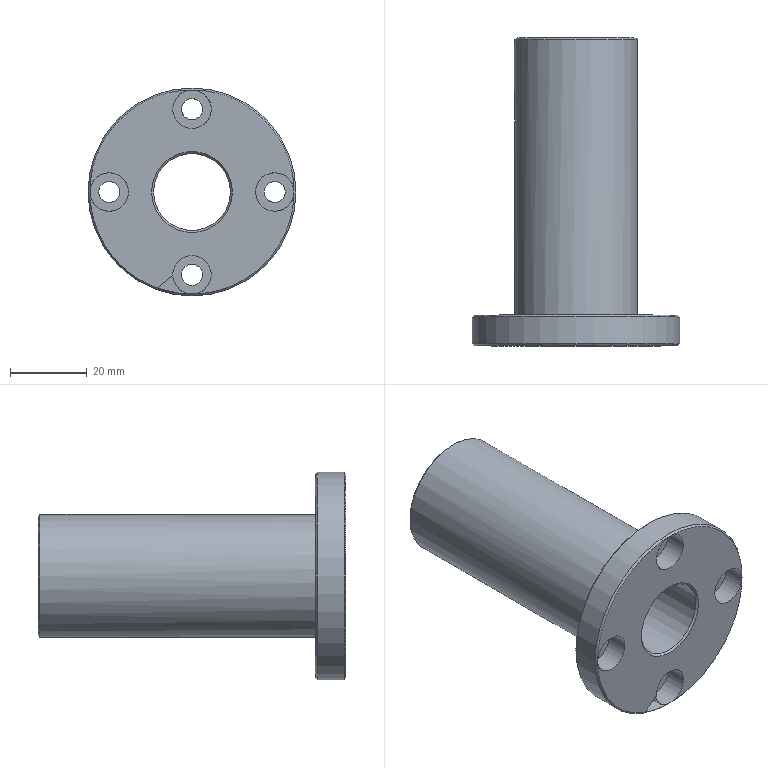Part | NX | 1 solid | 23 faces | box 54 x 80 x 54 mm | volume 49015 mm3 | cylinder 11 | plane 7 | cone 5 | commonest cylinder face diameters 5.5 x4 10 x4 20 x1 32 x1 54 x1
STEP:
#1=CARTESIAN_POINT('',(10.5,0.,0.));
#2=VERTEX_POINT('',#1);
#3=CARTESIAN_POINT('',(0.,0.,0.));
#4=DIRECTION('',(0.,-1.,0.));
#5=DIRECTION('',(1.,0.,0.));
#6=AXIS2_PLACEMENT_3D('',#3,#4,#5);
#7=CIRCLE('',#6,10.5);
#8=EDGE_CURVE('',#2,#2,#7,.F.);
#9=ORIENTED_EDGE('',*,*,#8,.T.);
#10=EDGE_LOOP('',(#9));
#11=FACE_BOUND('',#10,.T.);
#12=CARTESIAN_POINT('',(26.5,0.,0.));
#13=VERTEX_POINT('',#12);
#14=CARTESIAN_POINT('',(21.5,0.,0.));
#15=DIRECTION('',(0.,-1.,0.));
#16=DIRECTION('',(0.,0.,-1.));
#17=AXIS2_PLACEMENT_3D('',#14,#15,#16);
#18=CIRCLE('',#17,5.);
#19=EDGE_CURVE('',#13,#13,#18,.T.);
#20=ORIENTED_EDGE('',*,*,#19,.F.);
#21=CARTESIAN_POINT('',(0.,0.,26.5));
#22=VERTEX_POINT('',#21);
#23=CARTESIAN_POINT('',(0.,0.,0.));
#24=DIRECTION('',(0.,-1.,0.));
#25=DIRECTION('',(1.,0.,0.));
#26=AXIS2_PLACEMENT_3D('',#23,#24,#25);
#27=CIRCLE('',#26,26.5);
#28=EDGE_CURVE('',#13,#22,#27,.T.);
#29=ORIENTED_EDGE('',*,*,#28,.T.);
#30=CARTESIAN_POINT('',(0.,0.,21.5));
#31=DIRECTION('',(0.,-1.,0.));
#32=DIRECTION('',(0.,0.,-1.));
#33=AXIS2_PLACEMENT_3D('',#30,#31,#32);
#34=CIRCLE('',#33,5.);
#35=EDGE_CURVE('',#22,#22,#34,.T.);
#36=ORIENTED_EDGE('',*,*,#35,.F.);
#37=CARTESIAN_POINT('',(-26.5,0.,0.));
#38=VERTEX_POINT('',#37);
#39=CARTESIAN_POINT('',(0.,0.,0.));
#40=DIRECTION('',(0.,-1.,0.));
#41=DIRECTION('',(1.,0.,0.));
#42=AXIS2_PLACEMENT_3D('',#39,#40,#41);
#43=CIRCLE('',#42,26.5);
#44=EDGE_CURVE('',#22,#38,#43,.T.);
#45=ORIENTED_EDGE('',*,*,#44,.T.);
#46=CARTESIAN_POINT('',(-21.5,0.,0.));
#47=DIRECTION('',(0.,-1.,0.));
#48=DIRECTION('',(0.,0.,-1.));
#49=AXIS2_PLACEMENT_3D('',#46,#47,#48);
#50=CIRCLE('',#49,5.);
#51=EDGE_CURVE('',#38,#38,#50,.T.);
#52=ORIENTED_EDGE('',*,*,#51,.F.);
#53=CARTESIAN_POINT('',(0.,0.,-26.5));
#54=VERTEX_POINT('',#53);
#55=CARTESIAN_POINT('',(0.,0.,0.));
#56=DIRECTION('',(0.,-1.,0.));
#57=DIRECTION('',(1.,0.,0.));
#58=AXIS2_PLACEMENT_3D('',#55,#56,#57);
#59=CIRCLE('',#58,26.5);
#60=EDGE_CURVE('',#38,#54,#59,.T.);
#61=ORIENTED_EDGE('',*,*,#60,.T.);
#62=CARTESIAN_POINT('',(0.,0.,-21.5));
#63=DIRECTION('',(0.,-1.,0.));
#64=DIRECTION('',(0.,0.,-1.));
#65=AXIS2_PLACEMENT_3D('',#62,#63,#64);
#66=CIRCLE('',#65,5.);
#67=EDGE_CURVE('',#54,#54,#66,.T.);
#68=ORIENTED_EDGE('',*,*,#67,.F.);
#69=CARTESIAN_POINT('',(0.,0.,0.));
#70=DIRECTION('',(0.,-1.,0.));
#71=DIRECTION('',(1.,0.,0.));
#72=AXIS2_PLACEMENT_3D('',#69,#70,#71);
#73=CIRCLE('',#72,26.5);
#74=EDGE_CURVE('',#54,#13,#73,.T.);
#75=ORIENTED_EDGE('',*,*,#74,.T.);
#76=EDGE_LOOP('',(#20,#29,#36,#45,#52,#61,#68,#75));
#77=FACE_BOUND('',#76,.T.);
#78=CARTESIAN_POINT('',(10.,0.,0.));
#79=DIRECTION('',(0.,-1.,0.));
#80=DIRECTION('',(1.,0.,0.));
#81=AXIS2_PLACEMENT_3D('',#78,#79,#80);
#82=PLANE('',#81);
#83=ADVANCED_FACE('',(#11,#77),#82,.T.);
#84=CARTESIAN_POINT('',(-10.,79.5,0.));
#85=VERTEX_POINT('',#84);
#86=CARTESIAN_POINT('',(0.,79.5,0.));
#87=DIRECTION('',(0.,1.,0.));
#88=DIRECTION('',(-1.,0.,0.));
#89=AXIS2_PLACEMENT_3D('',#86,#87,#88);
#90=CIRCLE('',#89,10.);
#91=EDGE_CURVE('',#85,#85,#90,.T.);
#92=ORIENTED_EDGE('',*,*,#91,.T.);
#93=EDGE_LOOP('',(#92));
#94=FACE_BOUND('',#93,.T.);
#95=CARTESIAN_POINT('',(10.,0.5,0.));
#96=VERTEX_POINT('',#95);
#97=CARTESIAN_POINT('',(0.,0.5,0.));
#98=DIRECTION('',(0.,-1.,0.));
#99=DIRECTION('',(1.,0.,0.));
#100=AXIS2_PLACEMENT_3D('',#97,#98,#99);
#101=CIRCLE('',#100,10.);
#102=EDGE_CURVE('',#96,#96,#101,.T.);
#103=ORIENTED_EDGE('',*,*,#102,.T.);
#104=EDGE_LOOP('',(#103));
#105=FACE_BOUND('',#104,.T.);
#106=CARTESIAN_POINT('',(0.,-1000.,0.));
#107=DIRECTION('',(0.,-1.,0.));
#108=DIRECTION('',(1.,0.,0.));
#109=AXIS2_PLACEMENT_3D('',#106,#107,#108);
#110=CYLINDRICAL_SURFACE('',#109,10.);
#111=ADVANCED_FACE('',(#94,#105),#110,.F.);
#112=CARTESIAN_POINT('',(-10.5,80.,0.));
#113=VERTEX_POINT('',#112);
#114=CARTESIAN_POINT('',(0.,80.,0.));
#115=DIRECTION('',(0.,1.,0.));
#116=DIRECTION('',(-1.,0.,0.));
#117=AXIS2_PLACEMENT_3D('',#114,#115,#116);
#118=CIRCLE('',#117,10.5);
#119=EDGE_CURVE('',#113,#113,#118,.F.);
#120=ORIENTED_EDGE('',*,*,#119,.T.);
#121=EDGE_LOOP('',(#120));
#122=FACE_BOUND('',#121,.T.);
#123=CARTESIAN_POINT('',(-15.5,80.,0.));
#124=VERTEX_POINT('',#123);
#125=CARTESIAN_POINT('',(0.,80.,0.));
#126=DIRECTION('',(0.,1.,0.));
#127=DIRECTION('',(-1.,0.,0.));
#128=AXIS2_PLACEMENT_3D('',#125,#126,#127);
#129=CIRCLE('',#128,15.5);
#130=EDGE_CURVE('',#124,#124,#129,.T.);
#131=ORIENTED_EDGE('',*,*,#130,.T.);
#132=EDGE_LOOP('',(#131));
#133=FACE_BOUND('',#132,.T.);
#134=CARTESIAN_POINT('',(10.,80.,0.));
#135=DIRECTION('',(0.,1.,0.));
#136=DIRECTION('',(-1.,0.,0.));
#137=AXIS2_PLACEMENT_3D('',#134,#135,#136);
#138=PLANE('',#137);
#139=ADVANCED_FACE('',(#122,#133),#138,.T.);
#140=CARTESIAN_POINT('',(-16.,79.5,0.));
#141=VERTEX_POINT('',#140);
#142=CARTESIAN_POINT('',(0.,79.5,0.));
#143=DIRECTION('',(0.,1.,0.));
#144=DIRECTION('',(-1.,0.,0.));
#145=AXIS2_PLACEMENT_3D('',#142,#143,#144);
#146=CIRCLE('',#145,16.);
#147=EDGE_CURVE('',#141,#141,#146,.F.);
#148=ORIENTED_EDGE('',*,*,#147,.T.);
#149=EDGE_LOOP('',(#148));
#150=FACE_BOUND('',#149,.T.);
#151=CARTESIAN_POINT('',(16.,8.,0.));
#152=VERTEX_POINT('',#151);
#153=CARTESIAN_POINT('',(0.,8.,0.));
#154=DIRECTION('',(0.,-1.,0.));
#155=DIRECTION('',(1.,0.,0.));
#156=AXIS2_PLACEMENT_3D('',#153,#154,#155);
#157=CIRCLE('',#156,16.);
#158=EDGE_CURVE('',#152,#152,#157,.T.);
#159=ORIENTED_EDGE('',*,*,#158,.F.);
#160=EDGE_LOOP('',(#159));
#161=FACE_BOUND('',#160,.T.);
#162=CARTESIAN_POINT('',(0.,-1000.,0.));
#163=DIRECTION('',(0.,-1.,0.));
#164=DIRECTION('',(1.,0.,0.));
#165=AXIS2_PLACEMENT_3D('',#162,#163,#164);
#166=CYLINDRICAL_SURFACE('',#165,16.);
#167=ADVANCED_FACE('',(#150,#161),#166,.T.);
#168=CARTESIAN_POINT('',(-26.5,8.,0.));
#169=VERTEX_POINT('',#168);
#170=CARTESIAN_POINT('',(0.,8.,0.));
#171=DIRECTION('',(0.,1.,0.));
#172=DIRECTION('',(-1.,0.,0.));
#173=AXIS2_PLACEMENT_3D('',#170,#171,#172);
#174=CIRCLE('',#173,26.5);
#175=EDGE_CURVE('',#169,#169,#174,.T.);
#176=ORIENTED_EDGE('',*,*,#175,.T.);
#177=EDGE_LOOP('',(#176));
#178=FACE_BOUND('',#177,.T.);
#179=CARTESIAN_POINT('',(-24.25,8.,0.));
#180=VERTEX_POINT('',#179);
#181=CARTESIAN_POINT('',(-21.5,8.,0.));
#182=DIRECTION('',(0.,1.,0.));
#183=DIRECTION('',(-1.,0.,0.));
#184=AXIS2_PLACEMENT_3D('',#181,#182,#183);
#185=CIRCLE('',#184,2.75);
#186=EDGE_CURVE('',#180,#180,#185,.T.);
#187=ORIENTED_EDGE('',*,*,#186,.F.);
#188=EDGE_LOOP('',(#187));
#189=FACE_BOUND('',#188,.T.);
#190=CARTESIAN_POINT('',(-2.75,8.,21.5));
#191=VERTEX_POINT('',#190);
#192=CARTESIAN_POINT('',(0.,8.,21.5));
#193=DIRECTION('',(0.,1.,0.));
#194=DIRECTION('',(-1.,0.,0.));
#195=AXIS2_PLACEMENT_3D('',#192,#193,#194);
#196=CIRCLE('',#195,2.75);
#197=EDGE_CURVE('',#191,#191,#196,.T.);
#198=ORIENTED_EDGE('',*,*,#197,.F.);
#199=EDGE_LOOP('',(#198));
#200=FACE_BOUND('',#199,.T.);
#201=CARTESIAN_POINT('',(18.75,8.,0.));
#202=VERTEX_POINT('',#201);
#203=CARTESIAN_POINT('',(21.5,8.,0.));
#204=DIRECTION('',(0.,1.,0.));
#205=DIRECTION('',(-1.,0.,0.));
#206=AXIS2_PLACEMENT_3D('',#203,#204,#205);
#207=CIRCLE('',#206,2.75);
#208=EDGE_CURVE('',#202,#202,#207,.T.);
#209=ORIENTED_EDGE('',*,*,#208,.F.);
#210=EDGE_LOOP('',(#209));
#211=FACE_BOUND('',#210,.T.);
#212=CARTESIAN_POINT('',(-2.75,8.,-21.5));
#213=VERTEX_POINT('',#212);
#214=CARTESIAN_POINT('',(0.,8.,-21.5));
#215=DIRECTION('',(0.,1.,0.));
#216=DIRECTION('',(-1.,0.,0.));
#217=AXIS2_PLACEMENT_3D('',#214,#215,#216);
#218=CIRCLE('',#217,2.75);
#219=EDGE_CURVE('',#213,#213,#218,.T.);
#220=ORIENTED_EDGE('',*,*,#219,.F.);
#221=EDGE_LOOP('',(#220));
#222=FACE_BOUND('',#221,.T.);
#223=ORIENTED_EDGE('',*,*,#158,.T.);
#224=EDGE_LOOP('',(#223));
#225=FACE_BOUND('',#224,.T.);
#226=CARTESIAN_POINT('',(16.,8.,0.));
#227=DIRECTION('',(0.,1.,0.));
#228=DIRECTION('',(-1.,0.,0.));
#229=AXIS2_PLACEMENT_3D('',#226,#227,#228);
#230=PLANE('',#229);
#231=ADVANCED_FACE('',(#178,#189,#200,#211,#222,#225),#230,.T.);
#232=CARTESIAN_POINT('',(27.,0.5,0.));
#233=VERTEX_POINT('',#232);
#234=CARTESIAN_POINT('',(0.,0.5,0.));
#235=DIRECTION('',(0.,-1.,0.));
#236=DIRECTION('',(1.,0.,0.));
#237=AXIS2_PLACEMENT_3D('',#234,#235,#236);
#238=CIRCLE('',#237,27.);
#239=EDGE_CURVE('',#233,#233,#238,.F.);
#240=ORIENTED_EDGE('',*,*,#239,.T.);
#241=EDGE_LOOP('',(#240));
#242=FACE_BOUND('',#241,.T.);
#243=CARTESIAN_POINT('',(-27.,7.5,0.));
#244=VERTEX_POINT('',#243);
#245=CARTESIAN_POINT('',(0.,7.5,0.));
#246=DIRECTION('',(0.,1.,0.));
#247=DIRECTION('',(-1.,0.,0.));
#248=AXIS2_PLACEMENT_3D('',#245,#246,#247);
#249=CIRCLE('',#248,27.);
#250=EDGE_CURVE('',#244,#244,#249,.F.);
#251=ORIENTED_EDGE('',*,*,#250,.T.);
#252=EDGE_LOOP('',(#251));
#253=FACE_BOUND('',#252,.T.);
#254=CARTESIAN_POINT('',(0.,-1000.,0.));
#255=DIRECTION('',(0.,-1.,0.));
#256=DIRECTION('',(1.,0.,0.));
#257=AXIS2_PLACEMENT_3D('',#254,#255,#256);
#258=CYLINDRICAL_SURFACE('',#257,27.);
#259=ADVANCED_FACE('',(#242,#253),#258,.T.);
#260=ORIENTED_EDGE('',*,*,#219,.T.);
#261=EDGE_LOOP('',(#260));
#262=FACE_BOUND('',#261,.T.);
#263=CARTESIAN_POINT('',(0.,5.7,-24.25));
#264=VERTEX_POINT('',#263);
#265=CARTESIAN_POINT('',(0.,5.7,-21.5));
#266=DIRECTION('',(0.,-1.,0.));
#267=DIRECTION('',(0.,0.,-1.));
#268=AXIS2_PLACEMENT_3D('',#265,#266,#267);
#269=CIRCLE('',#268,2.75);
#270=EDGE_CURVE('',#264,#264,#269,.T.);
#271=ORIENTED_EDGE('',*,*,#270,.T.);
#272=EDGE_LOOP('',(#271));
#273=FACE_BOUND('',#272,.T.);
#274=CARTESIAN_POINT('',(0.,0.,-21.5));
#275=DIRECTION('',(0.,-1.,0.));
#276=DIRECTION('',(0.,0.,-1.));
#277=AXIS2_PLACEMENT_3D('',#274,#275,#276);
#278=CYLINDRICAL_SURFACE('',#277,2.75);
#279=ADVANCED_FACE('',(#262,#273),#278,.F.);
#280=ORIENTED_EDGE('',*,*,#270,.F.);
#281=EDGE_LOOP('',(#280));
#282=FACE_BOUND('',#281,.T.);
#283=CARTESIAN_POINT('',(0.,5.7,-26.5));
#284=VERTEX_POINT('',#283);
#285=CARTESIAN_POINT('',(0.,5.7,-21.5));
#286=DIRECTION('',(0.,-1.,0.));
#287=DIRECTION('',(0.,0.,-1.));
#288=AXIS2_PLACEMENT_3D('',#285,#286,#287);
#289=CIRCLE('',#288,5.);
#290=EDGE_CURVE('',#284,#284,#289,.T.);
#291=ORIENTED_EDGE('',*,*,#290,.T.);
#292=EDGE_LOOP('',(#291));
#293=FACE_BOUND('',#292,.T.);
#294=CARTESIAN_POINT('',(2.75,5.7,-21.5));
#295=DIRECTION('',(0.,1.,0.));
#296=DIRECTION('',(0.,0.,1.));
#297=AXIS2_PLACEMENT_3D('',#294,#295,#296);
#298=PLANE('',#297);
#299=ADVANCED_FACE('',(#282,#293),#298,.F.);
#300=ORIENTED_EDGE('',*,*,#290,.F.);
#301=EDGE_LOOP('',(#300));
#302=FACE_BOUND('',#301,.T.);
#303=ORIENTED_EDGE('',*,*,#67,.T.);
#304=EDGE_LOOP('',(#303));
#305=FACE_BOUND('',#304,.T.);
#306=CARTESIAN_POINT('',(0.,0.,-21.5));
#307=DIRECTION('',(0.,-1.,0.));
#308=DIRECTION('',(0.,0.,-1.));
#309=AXIS2_PLACEMENT_3D('',#306,#307,#308);
#310=CYLINDRICAL_SURFACE('',#309,5.);
#311=ADVANCED_FACE('',(#302,#305),#310,.F.);
#312=ORIENTED_EDGE('',*,*,#208,.T.);
#313=EDGE_LOOP('',(#312));
#314=FACE_BOUND('',#313,.T.);
#315=CARTESIAN_POINT('',(21.5,5.7,-2.75));
#316=VERTEX_POINT('',#315);
#317=CARTESIAN_POINT('',(21.5,5.7,0.));
#318=DIRECTION('',(0.,-1.,0.));
#319=DIRECTION('',(0.,0.,-1.));
#320=AXIS2_PLACEMENT_3D('',#317,#318,#319);
#321=CIRCLE('',#320,2.75);
#322=EDGE_CURVE('',#316,#316,#321,.T.);
#323=ORIENTED_EDGE('',*,*,#322,.T.);
#324=EDGE_LOOP('',(#323));
#325=FACE_BOUND('',#324,.T.);
#326=CARTESIAN_POINT('',(21.5,0.,0.));
#327=DIRECTION('',(0.,-1.,0.));
#328=DIRECTION('',(0.,0.,-1.));
#329=AXIS2_PLACEMENT_3D('',#326,#327,#328);
#330=CYLINDRICAL_SURFACE('',#329,2.75);
#331=ADVANCED_FACE('',(#314,#325),#330,.F.);
#332=ORIENTED_EDGE('',*,*,#322,.F.);
#333=EDGE_LOOP('',(#332));
#334=FACE_BOUND('',#333,.T.);
#335=CARTESIAN_POINT('',(21.5,5.7,-5.));
#336=VERTEX_POINT('',#335);
#337=CARTESIAN_POINT('',(21.5,5.7,0.));
#338=DIRECTION('',(0.,-1.,0.));
#339=DIRECTION('',(0.,0.,-1.));
#340=AXIS2_PLACEMENT_3D('',#337,#338,#339);
#341=CIRCLE('',#340,5.);
#342=EDGE_CURVE('',#336,#336,#341,.T.);
#343=ORIENTED_EDGE('',*,*,#342,.T.);
#344=EDGE_LOOP('',(#343));
#345=FACE_BOUND('',#344,.T.);
#346=CARTESIAN_POINT('',(24.25,5.7,0.));
#347=DIRECTION('',(0.,1.,0.));
#348=DIRECTION('',(0.,0.,1.));
#349=AXIS2_PLACEMENT_3D('',#346,#347,#348);
#350=PLANE('',#349);
#351=ADVANCED_FACE('',(#334,#345),#350,.F.);
#352=ORIENTED_EDGE('',*,*,#342,.F.);
#353=EDGE_LOOP('',(#352));
#354=FACE_BOUND('',#353,.T.);
#355=ORIENTED_EDGE('',*,*,#19,.T.);
#356=EDGE_LOOP('',(#355));
#357=FACE_BOUND('',#356,.T.);
#358=CARTESIAN_POINT('',(21.5,0.,0.));
#359=DIRECTION('',(0.,-1.,0.));
#360=DIRECTION('',(0.,0.,-1.));
#361=AXIS2_PLACEMENT_3D('',#358,#359,#360);
#362=CYLINDRICAL_SURFACE('',#361,5.);
#363=ADVANCED_FACE('',(#354,#357),#362,.F.);
#364=ORIENTED_EDGE('',*,*,#197,.T.);
#365=EDGE_LOOP('',(#364));
#366=FACE_BOUND('',#365,.T.);
#367=CARTESIAN_POINT('',(0.,5.7,18.75));
#368=VERTEX_POINT('',#367);
#369=CARTESIAN_POINT('',(0.,5.7,21.5));
#370=DIRECTION('',(0.,-1.,0.));
#371=DIRECTION('',(0.,0.,-1.));
#372=AXIS2_PLACEMENT_3D('',#369,#370,#371);
#373=CIRCLE('',#372,2.75);
#374=EDGE_CURVE('',#368,#368,#373,.T.);
#375=ORIENTED_EDGE('',*,*,#374,.T.);
#376=EDGE_LOOP('',(#375));
#377=FACE_BOUND('',#376,.T.);
#378=CARTESIAN_POINT('',(0.,0.,21.5));
#379=DIRECTION('',(0.,-1.,0.));
#380=DIRECTION('',(0.,0.,-1.));
#381=AXIS2_PLACEMENT_3D('',#378,#379,#380);
#382=CYLINDRICAL_SURFACE('',#381,2.75);
#383=ADVANCED_FACE('',(#366,#377),#382,.F.);
#384=ORIENTED_EDGE('',*,*,#374,.F.);
#385=EDGE_LOOP('',(#384));
#386=FACE_BOUND('',#385,.T.);
#387=CARTESIAN_POINT('',(0.,5.7,16.5));
#388=VERTEX_POINT('',#387);
#389=CARTESIAN_POINT('',(0.,5.7,21.5));
#390=DIRECTION('',(0.,-1.,0.));
#391=DIRECTION('',(0.,0.,-1.));
#392=AXIS2_PLACEMENT_3D('',#389,#390,#391);
#393=CIRCLE('',#392,5.);
#394=EDGE_CURVE('',#388,#388,#393,.T.);
#395=ORIENTED_EDGE('',*,*,#394,.T.);
#396=EDGE_LOOP('',(#395));
#397=FACE_BOUND('',#396,.T.);
#398=CARTESIAN_POINT('',(2.75,5.7,21.5));
#399=DIRECTION('',(0.,1.,0.));
#400=DIRECTION('',(0.,0.,1.));
#401=AXIS2_PLACEMENT_3D('',#398,#399,#400);
#402=PLANE('',#401);
#403=ADVANCED_FACE('',(#386,#397),#402,.F.);
#404=ORIENTED_EDGE('',*,*,#394,.F.);
#405=EDGE_LOOP('',(#404));
#406=FACE_BOUND('',#405,.T.);
#407=ORIENTED_EDGE('',*,*,#35,.T.);
#408=EDGE_LOOP('',(#407));
#409=FACE_BOUND('',#408,.T.);
#410=CARTESIAN_POINT('',(0.,0.,21.5));
#411=DIRECTION('',(0.,-1.,0.));
#412=DIRECTION('',(0.,0.,-1.));
#413=AXIS2_PLACEMENT_3D('',#410,#411,#412);
#414=CYLINDRICAL_SURFACE('',#413,5.);
#415=ADVANCED_FACE('',(#406,#409),#414,.F.);
#416=ORIENTED_EDGE('',*,*,#186,.T.);
#417=EDGE_LOOP('',(#416));
#418=FACE_BOUND('',#417,.T.);
#419=CARTESIAN_POINT('',(-21.5,5.7,-2.75));
#420=VERTEX_POINT('',#419);
#421=CARTESIAN_POINT('',(-21.5,5.7,0.));
#422=DIRECTION('',(0.,-1.,0.));
#423=DIRECTION('',(0.,0.,-1.));
#424=AXIS2_PLACEMENT_3D('',#421,#422,#423);
#425=CIRCLE('',#424,2.75);
#426=EDGE_CURVE('',#420,#420,#425,.T.);
#427=ORIENTED_EDGE('',*,*,#426,.T.);
#428=EDGE_LOOP('',(#427));
#429=FACE_BOUND('',#428,.T.);
#430=CARTESIAN_POINT('',(-21.5,0.,0.));
#431=DIRECTION('',(0.,-1.,0.));
#432=DIRECTION('',(0.,0.,-1.));
#433=AXIS2_PLACEMENT_3D('',#430,#431,#432);
#434=CYLINDRICAL_SURFACE('',#433,2.75);
#435=ADVANCED_FACE('',(#418,#429),#434,.F.);
#436=ORIENTED_EDGE('',*,*,#426,.F.);
#437=EDGE_LOOP('',(#436));
#438=FACE_BOUND('',#437,.T.);
#439=CARTESIAN_POINT('',(-21.5,5.7,-5.));
#440=VERTEX_POINT('',#439);
#441=CARTESIAN_POINT('',(-21.5,5.7,0.));
#442=DIRECTION('',(0.,-1.,0.));
#443=DIRECTION('',(0.,0.,-1.));
#444=AXIS2_PLACEMENT_3D('',#441,#442,#443);
#445=CIRCLE('',#444,5.);
#446=EDGE_CURVE('',#440,#440,#445,.T.);
#447=ORIENTED_EDGE('',*,*,#446,.T.);
#448=EDGE_LOOP('',(#447));
#449=FACE_BOUND('',#448,.T.);
#450=CARTESIAN_POINT('',(-18.75,5.7,0.));
#451=DIRECTION('',(0.,1.,0.));
#452=DIRECTION('',(0.,0.,1.));
#453=AXIS2_PLACEMENT_3D('',#450,#451,#452);
#454=PLANE('',#453);
#455=ADVANCED_FACE('',(#438,#449),#454,.F.);
#456=ORIENTED_EDGE('',*,*,#446,.F.);
#457=EDGE_LOOP('',(#456));
#458=FACE_BOUND('',#457,.T.);
#459=ORIENTED_EDGE('',*,*,#51,.T.);
#460=EDGE_LOOP('',(#459));
#461=FACE_BOUND('',#460,.T.);
#462=CARTESIAN_POINT('',(-21.5,0.,0.));
#463=DIRECTION('',(0.,-1.,0.));
#464=DIRECTION('',(0.,0.,-1.));
#465=AXIS2_PLACEMENT_3D('',#462,#463,#464);
#466=CYLINDRICAL_SURFACE('',#465,5.);
#467=ADVANCED_FACE('',(#458,#461),#466,.F.);
#468=ORIENTED_EDGE('',*,*,#91,.F.);
#469=EDGE_LOOP('',(#468));
#470=FACE_BOUND('',#469,.T.);
#471=ORIENTED_EDGE('',*,*,#119,.F.);
#472=EDGE_LOOP('',(#471));
#473=FACE_BOUND('',#472,.T.);
#474=CARTESIAN_POINT('',(0.,80.,0.));
#475=DIRECTION('',(0.,1.,0.));
#476=DIRECTION('',(-1.,0.,0.));
#477=AXIS2_PLACEMENT_3D('',#474,#475,#476);
#478=CONICAL_SURFACE('',#477,10.5,0.7854);
#479=ADVANCED_FACE('',(#470,#473),#478,.F.);
#480=ORIENTED_EDGE('',*,*,#8,.F.);
#481=EDGE_LOOP('',(#480));
#482=FACE_BOUND('',#481,.T.);
#483=ORIENTED_EDGE('',*,*,#102,.F.);
#484=EDGE_LOOP('',(#483));
#485=FACE_BOUND('',#484,.T.);
#486=CARTESIAN_POINT('',(0.,0.5,0.));
#487=DIRECTION('',(0.,-1.,0.));
#488=DIRECTION('',(1.,0.,0.));
#489=AXIS2_PLACEMENT_3D('',#486,#487,#488);
#490=CONICAL_SURFACE('',#489,10.,0.7854);
#491=ADVANCED_FACE('',(#482,#485),#490,.F.);
#492=ORIENTED_EDGE('',*,*,#130,.F.);
#493=EDGE_LOOP('',(#492));
#494=FACE_BOUND('',#493,.T.);
#495=ORIENTED_EDGE('',*,*,#147,.F.);
#496=EDGE_LOOP('',(#495));
#497=FACE_BOUND('',#496,.T.);
#498=CARTESIAN_POINT('',(0.,79.5,0.));
#499=DIRECTION('',(0.,-1.,0.));
#500=DIRECTION('',(1.,0.,0.));
#501=AXIS2_PLACEMENT_3D('',#498,#499,#500);
#502=CONICAL_SURFACE('',#501,16.,0.7854);
#503=ADVANCED_FACE('',(#494,#497),#502,.T.);
#504=ORIENTED_EDGE('',*,*,#239,.F.);
#505=EDGE_LOOP('',(#504));
#506=FACE_BOUND('',#505,.T.);
#507=ORIENTED_EDGE('',*,*,#44,.F.);
#508=ORIENTED_EDGE('',*,*,#28,.F.);
#509=ORIENTED_EDGE('',*,*,#74,.F.);
#510=ORIENTED_EDGE('',*,*,#60,.F.);
#511=EDGE_LOOP('',(#507,#508,#509,#510));
#512=FACE_BOUND('',#511,.T.);
#513=CARTESIAN_POINT('',(0.,0.,0.));
#514=DIRECTION('',(0.,1.,0.));
#515=DIRECTION('',(-1.,0.,0.));
#516=AXIS2_PLACEMENT_3D('',#513,#514,#515);
#517=CONICAL_SURFACE('',#516,26.5,0.7854);
#518=ADVANCED_FACE('',(#506,#512),#517,.T.);
#519=ORIENTED_EDGE('',*,*,#175,.F.);
#520=EDGE_LOOP('',(#519));
#521=FACE_BOUND('',#520,.T.);
#522=ORIENTED_EDGE('',*,*,#250,.F.);
#523=EDGE_LOOP('',(#522));
#524=FACE_BOUND('',#523,.T.);
#525=CARTESIAN_POINT('',(0.,7.5,0.));
#526=DIRECTION('',(0.,-1.,0.));
#527=DIRECTION('',(1.,0.,0.));
#528=AXIS2_PLACEMENT_3D('',#525,#526,#527);
#529=CONICAL_SURFACE('',#528,27.,0.7854);
#530=ADVANCED_FACE('',(#521,#524),#529,.T.);
#531=CLOSED_SHELL('',(#83,#111,#139,#167,#231,#259,#279,#299,#311,#331,#351,#363,#383,#403,#415,#435,#455,#467,#479,#491,#503,#518,#530));
#532=MANIFOLD_SOLID_BREP('',#531);
#533=(LENGTH_UNIT()NAMED_UNIT(*)SI_UNIT(.MILLI.,.METRE.));
#534=UNCERTAINTY_MEASURE_WITH_UNIT(LENGTH_MEASURE(0.00001),#533,'','');
#535=(NAMED_UNIT(*)PLANE_ANGLE_UNIT()SI_UNIT($,.RADIAN.));
#536=(NAMED_UNIT(*)SI_UNIT($,.STERADIAN.)SOLID_ANGLE_UNIT());
#537=(GEOMETRIC_REPRESENTATION_CONTEXT(3)GLOBAL_UNCERTAINTY_ASSIGNED_CONTEXT((#534))GLOBAL_UNIT_ASSIGNED_CONTEXT((#533,#535,#536))REPRESENTATION_CONTEXT('',''));
#538=ADVANCED_BREP_SHAPE_REPRESENTATION('',(#532),#537);